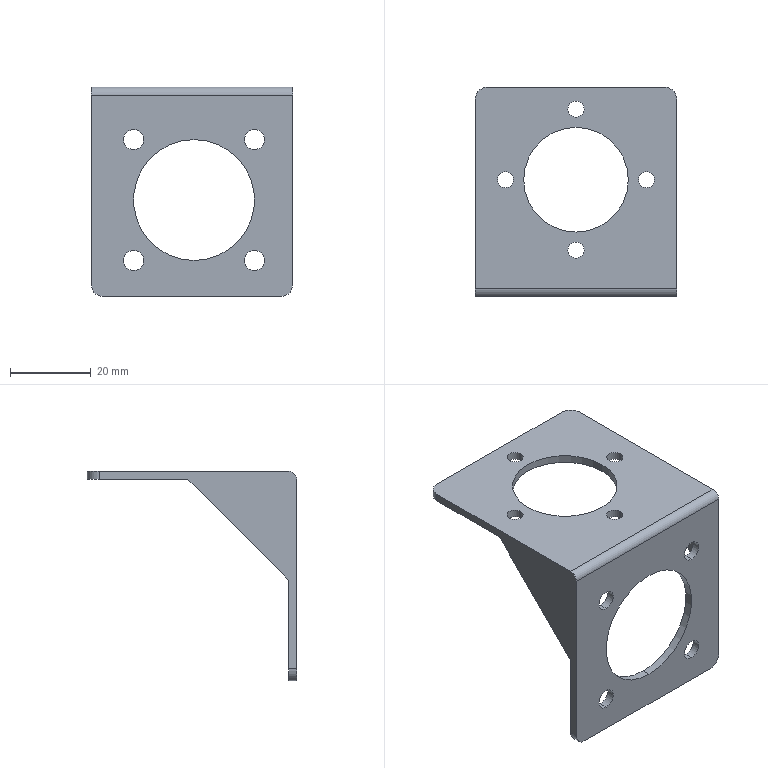Part | SolidWorks | features BaseBody 1 | 1 solid | 37 faces | box 50 x 52 x 52 mm | volume 8658 mm3 | cylinder 25 | plane 12 | commonest cylinder face diameters 4 x9 5 x8 6 x4 26 x2 30 x2
STEP:
#1=CARTESIAN_POINT('',(55.639,29.003,-82.334));
#2=VERTEX_POINT('',#1);
#3=CARTESIAN_POINT('',(51.639,29.003,-82.334));
#4=VERTEX_POINT('',#3);
#5=CARTESIAN_POINT('',(53.639,29.003,-82.334));
#6=DIRECTION('',(0.,0.,-1.));
#7=DIRECTION('',(-1.,0.,0.));
#8=AXIS2_PLACEMENT_3D('',#5,#6,#7);
#9=CIRCLE('',#8,2.);
#10=EDGE_CURVE('',#2,#4,#9,.T.);
#11=ORIENTED_EDGE('',*,*,#10,.F.);
#12=CARTESIAN_POINT('',(55.639,29.003,-84.334));
#13=VERTEX_POINT('',#12);
#14=CARTESIAN_POINT('',(55.639,29.003,-82.334));
#15=DIRECTION('',(0.,0.,-1.));
#16=VECTOR('',#15,1000.);
#17=LINE('',#14,#16);
#18=EDGE_CURVE('',#2,#13,#17,.T.);
#19=ORIENTED_EDGE('',*,*,#18,.T.);
#20=CARTESIAN_POINT('',(51.639,29.003,-84.334));
#21=VERTEX_POINT('',#20);
#22=CARTESIAN_POINT('',(53.639,29.003,-84.334));
#23=DIRECTION('',(0.,0.,1.));
#24=DIRECTION('',(-1.,0.,0.));
#25=AXIS2_PLACEMENT_3D('',#22,#23,#24);
#26=CIRCLE('',#25,2.);
#27=EDGE_CURVE('',#21,#13,#26,.T.);
#28=ORIENTED_EDGE('',*,*,#27,.F.);
#29=CARTESIAN_POINT('',(51.639,29.003,-82.334));
#30=DIRECTION('',(0.,0.,-1.));
#31=VECTOR('',#30,1000.);
#32=LINE('',#29,#31);
#33=EDGE_CURVE('',#4,#21,#32,.T.);
#34=ORIENTED_EDGE('',*,*,#33,.F.);
#35=EDGE_LOOP('',(#11,#19,#28,#34));
#36=FACE_OUTER_BOUND('',#35,.T.);
#37=CARTESIAN_POINT('',(53.639,29.003,-82.334));
#38=DIRECTION('',(0.,0.,-1.));
#39=DIRECTION('',(-1.,0.,0.));
#40=AXIS2_PLACEMENT_3D('',#37,#38,#39);
#41=CYLINDRICAL_SURFACE('',#40,2.);
#42=ADVANCED_FACE('',(#36),#41,.F.);
#43=CARTESIAN_POINT('',(84.139,29.003,-82.334));
#44=VERTEX_POINT('',#43);
#45=CARTESIAN_POINT('',(58.139,29.003,-82.334));
#46=VERTEX_POINT('',#45);
#47=CARTESIAN_POINT('',(71.139,29.003,-82.334));
#48=DIRECTION('',(0.,0.,-1.));
#49=DIRECTION('',(-1.,0.,0.));
#50=AXIS2_PLACEMENT_3D('',#47,#48,#49);
#51=CIRCLE('',#50,13.);
#52=EDGE_CURVE('',#44,#46,#51,.T.);
#53=ORIENTED_EDGE('',*,*,#52,.F.);
#54=CARTESIAN_POINT('',(84.139,29.003,-84.334));
#55=VERTEX_POINT('',#54);
#56=CARTESIAN_POINT('',(84.139,29.003,-82.334));
#57=DIRECTION('',(0.,0.,-1.));
#58=VECTOR('',#57,1000.);
#59=LINE('',#56,#58);
#60=EDGE_CURVE('',#44,#55,#59,.T.);
#61=ORIENTED_EDGE('',*,*,#60,.T.);
#62=CARTESIAN_POINT('',(58.139,29.003,-84.334));
#63=VERTEX_POINT('',#62);
#64=CARTESIAN_POINT('',(71.139,29.003,-84.334));
#65=DIRECTION('',(0.,0.,1.));
#66=DIRECTION('',(-1.,0.,0.));
#67=AXIS2_PLACEMENT_3D('',#64,#65,#66);
#68=CIRCLE('',#67,13.);
#69=EDGE_CURVE('',#63,#55,#68,.T.);
#70=ORIENTED_EDGE('',*,*,#69,.F.);
#71=CARTESIAN_POINT('',(58.139,29.003,-82.334));
#72=DIRECTION('',(0.,0.,-1.));
#73=VECTOR('',#72,1000.);
#74=LINE('',#71,#73);
#75=EDGE_CURVE('',#46,#63,#74,.T.);
#76=ORIENTED_EDGE('',*,*,#75,.F.);
#77=EDGE_LOOP('',(#53,#61,#70,#76));
#78=FACE_OUTER_BOUND('',#77,.T.);
#79=CARTESIAN_POINT('',(71.139,29.003,-82.334));
#80=DIRECTION('',(0.,0.,-1.));
#81=DIRECTION('',(-1.,0.,0.));
#82=AXIS2_PLACEMENT_3D('',#79,#80,#81);
#83=CYLINDRICAL_SURFACE('',#82,13.);
#84=ADVANCED_FACE('',(#78),#83,.F.);
#85=CARTESIAN_POINT('',(90.639,29.003,-82.334));
#86=VERTEX_POINT('',#85);
#87=CARTESIAN_POINT('',(86.639,29.003,-82.334));
#88=VERTEX_POINT('',#87);
#89=CARTESIAN_POINT('',(88.639,29.003,-82.334));
#90=DIRECTION('',(0.,0.,-1.));
#91=DIRECTION('',(-1.,0.,0.));
#92=AXIS2_PLACEMENT_3D('',#89,#90,#91);
#93=CIRCLE('',#92,2.);
#94=EDGE_CURVE('',#86,#88,#93,.T.);
#95=ORIENTED_EDGE('',*,*,#94,.F.);
#96=CARTESIAN_POINT('',(90.639,29.003,-84.334));
#97=VERTEX_POINT('',#96);
#98=CARTESIAN_POINT('',(90.639,29.003,-82.334));
#99=DIRECTION('',(0.,0.,-1.));
#100=VECTOR('',#99,1000.);
#101=LINE('',#98,#100);
#102=EDGE_CURVE('',#86,#97,#101,.T.);
#103=ORIENTED_EDGE('',*,*,#102,.T.);
#104=CARTESIAN_POINT('',(86.639,29.003,-84.334));
#105=VERTEX_POINT('',#104);
#106=CARTESIAN_POINT('',(88.639,29.003,-84.334));
#107=DIRECTION('',(0.,0.,1.));
#108=DIRECTION('',(-1.,0.,0.));
#109=AXIS2_PLACEMENT_3D('',#106,#107,#108);
#110=CIRCLE('',#109,2.);
#111=EDGE_CURVE('',#105,#97,#110,.T.);
#112=ORIENTED_EDGE('',*,*,#111,.F.);
#113=CARTESIAN_POINT('',(86.639,29.003,-82.334));
#114=DIRECTION('',(0.,0.,-1.));
#115=VECTOR('',#114,1000.);
#116=LINE('',#113,#115);
#117=EDGE_CURVE('',#88,#105,#116,.T.);
#118=ORIENTED_EDGE('',*,*,#117,.F.);
#119=EDGE_LOOP('',(#95,#103,#112,#118));
#120=FACE_OUTER_BOUND('',#119,.T.);
#121=CARTESIAN_POINT('',(88.639,29.003,-82.334));
#122=DIRECTION('',(0.,0.,-1.));
#123=DIRECTION('',(-1.,0.,0.));
#124=AXIS2_PLACEMENT_3D('',#121,#122,#123);
#125=CYLINDRICAL_SURFACE('',#124,2.);
#126=ADVANCED_FACE('',(#120),#125,.F.);
#127=CARTESIAN_POINT('',(73.139,11.503,-82.334));
#128=VERTEX_POINT('',#127);
#129=CARTESIAN_POINT('',(69.139,11.503,-82.334));
#130=VERTEX_POINT('',#129);
#131=CARTESIAN_POINT('',(71.139,11.503,-82.334));
#132=DIRECTION('',(0.,0.,-1.));
#133=DIRECTION('',(-1.,0.,0.));
#134=AXIS2_PLACEMENT_3D('',#131,#132,#133);
#135=CIRCLE('',#134,2.);
#136=EDGE_CURVE('',#128,#130,#135,.T.);
#137=ORIENTED_EDGE('',*,*,#136,.F.);
#138=CARTESIAN_POINT('',(73.139,11.503,-84.334));
#139=VERTEX_POINT('',#138);
#140=CARTESIAN_POINT('',(73.139,11.503,-82.334));
#141=DIRECTION('',(0.,0.,-1.));
#142=VECTOR('',#141,1000.);
#143=LINE('',#140,#142);
#144=EDGE_CURVE('',#128,#139,#143,.T.);
#145=ORIENTED_EDGE('',*,*,#144,.T.);
#146=CARTESIAN_POINT('',(69.139,11.503,-84.334));
#147=VERTEX_POINT('',#146);
#148=CARTESIAN_POINT('',(71.139,11.503,-84.334));
#149=DIRECTION('',(0.,0.,1.));
#150=DIRECTION('',(-1.,0.,0.));
#151=AXIS2_PLACEMENT_3D('',#148,#149,#150);
#152=CIRCLE('',#151,2.);
#153=EDGE_CURVE('',#147,#139,#152,.T.);
#154=ORIENTED_EDGE('',*,*,#153,.F.);
#155=CARTESIAN_POINT('',(69.139,11.503,-82.334));
#156=DIRECTION('',(0.,0.,-1.));
#157=VECTOR('',#156,1000.);
#158=LINE('',#155,#157);
#159=EDGE_CURVE('',#130,#147,#158,.T.);
#160=ORIENTED_EDGE('',*,*,#159,.F.);
#161=EDGE_LOOP('',(#137,#145,#154,#160));
#162=FACE_OUTER_BOUND('',#161,.T.);
#163=CARTESIAN_POINT('',(71.139,11.503,-82.334));
#164=DIRECTION('',(0.,0.,-1.));
#165=DIRECTION('',(-1.,0.,0.));
#166=AXIS2_PLACEMENT_3D('',#163,#164,#165);
#167=CYLINDRICAL_SURFACE('',#166,2.);
#168=ADVANCED_FACE('',(#162),#167,.F.);
#169=CARTESIAN_POINT('',(73.139,46.503,-82.334));
#170=VERTEX_POINT('',#169);
#171=CARTESIAN_POINT('',(69.139,46.503,-82.334));
#172=VERTEX_POINT('',#171);
#173=CARTESIAN_POINT('',(71.139,46.503,-82.334));
#174=DIRECTION('',(0.,0.,-1.));
#175=DIRECTION('',(-1.,0.,0.));
#176=AXIS2_PLACEMENT_3D('',#173,#174,#175);
#177=CIRCLE('',#176,2.);
#178=EDGE_CURVE('',#170,#172,#177,.T.);
#179=ORIENTED_EDGE('',*,*,#178,.F.);
#180=CARTESIAN_POINT('',(73.139,46.503,-84.334));
#181=VERTEX_POINT('',#180);
#182=CARTESIAN_POINT('',(73.139,46.503,-82.334));
#183=DIRECTION('',(0.,0.,-1.));
#184=VECTOR('',#183,1000.);
#185=LINE('',#182,#184);
#186=EDGE_CURVE('',#170,#181,#185,.T.);
#187=ORIENTED_EDGE('',*,*,#186,.T.);
#188=CARTESIAN_POINT('',(69.139,46.503,-84.334));
#189=VERTEX_POINT('',#188);
#190=CARTESIAN_POINT('',(71.139,46.503,-84.334));
#191=DIRECTION('',(0.,0.,1.));
#192=DIRECTION('',(-1.,0.,0.));
#193=AXIS2_PLACEMENT_3D('',#190,#191,#192);
#194=CIRCLE('',#193,2.);
#195=EDGE_CURVE('',#189,#181,#194,.T.);
#196=ORIENTED_EDGE('',*,*,#195,.F.);
#197=CARTESIAN_POINT('',(69.139,46.503,-82.334));
#198=DIRECTION('',(0.,0.,-1.));
#199=VECTOR('',#198,1000.);
#200=LINE('',#197,#199);
#201=EDGE_CURVE('',#172,#189,#200,.T.);
#202=ORIENTED_EDGE('',*,*,#201,.F.);
#203=EDGE_LOOP('',(#179,#187,#196,#202));
#204=FACE_OUTER_BOUND('',#203,.T.);
#205=CARTESIAN_POINT('',(71.139,46.503,-82.334));
#206=DIRECTION('',(0.,0.,-1.));
#207=DIRECTION('',(-1.,0.,0.));
#208=AXIS2_PLACEMENT_3D('',#205,#206,#207);
#209=CYLINDRICAL_SURFACE('',#208,2.);
#210=ADVANCED_FACE('',(#204),#209,.F.);
#211=CARTESIAN_POINT('',(56.639,2.,-122.834));
#212=VERTEX_POINT('',#211);
#213=CARTESIAN_POINT('',(56.639,2.,-127.834));
#214=VERTEX_POINT('',#213);
#215=CARTESIAN_POINT('',(56.639,2.,-125.334));
#216=DIRECTION('',(0.,-1.,0.));
#217=DIRECTION('',(0.,0.,-1.));
#218=AXIS2_PLACEMENT_3D('',#215,#216,#217);
#219=CIRCLE('',#218,2.5);
#220=EDGE_CURVE('',#212,#214,#219,.T.);
#221=ORIENTED_EDGE('',*,*,#220,.F.);
#222=CARTESIAN_POINT('',(56.639,0.,-122.834));
#223=VERTEX_POINT('',#222);
#224=CARTESIAN_POINT('',(56.639,2.,-122.834));
#225=DIRECTION('',(0.,-1.,0.));
#226=VECTOR('',#225,1000.);
#227=LINE('',#224,#226);
#228=EDGE_CURVE('',#212,#223,#227,.T.);
#229=ORIENTED_EDGE('',*,*,#228,.T.);
#230=CARTESIAN_POINT('',(56.639,0.,-127.834));
#231=VERTEX_POINT('',#230);
#232=CARTESIAN_POINT('',(56.639,0.,-125.334));
#233=DIRECTION('',(0.,-1.,0.));
#234=DIRECTION('',(0.,0.,-1.));
#235=AXIS2_PLACEMENT_3D('',#232,#233,#234);
#236=CIRCLE('',#235,2.5);
#237=EDGE_CURVE('',#223,#231,#236,.T.);
#238=ORIENTED_EDGE('',*,*,#237,.T.);
#239=CARTESIAN_POINT('',(56.639,2.,-127.834));
#240=DIRECTION('',(0.,-1.,0.));
#241=VECTOR('',#240,1000.);
#242=LINE('',#239,#241);
#243=EDGE_CURVE('',#214,#231,#242,.T.);
#244=ORIENTED_EDGE('',*,*,#243,.F.);
#245=EDGE_LOOP('',(#221,#229,#238,#244));
#246=FACE_OUTER_BOUND('',#245,.T.);
#247=CARTESIAN_POINT('',(56.639,2.,-125.334));
#248=DIRECTION('',(0.,-1.,0.));
#249=DIRECTION('',(0.,0.,-1.));
#250=AXIS2_PLACEMENT_3D('',#247,#248,#249);
#251=CYLINDRICAL_SURFACE('',#250,2.5);
#252=ADVANCED_FACE('',(#246),#251,.F.);
#253=CARTESIAN_POINT('',(86.639,2.,-122.834));
#254=VERTEX_POINT('',#253);
#255=CARTESIAN_POINT('',(86.639,2.,-127.834));
#256=VERTEX_POINT('',#255);
#257=CARTESIAN_POINT('',(86.639,2.,-125.334));
#258=DIRECTION('',(0.,-1.,0.));
#259=DIRECTION('',(0.,0.,-1.));
#260=AXIS2_PLACEMENT_3D('',#257,#258,#259);
#261=CIRCLE('',#260,2.5);
#262=EDGE_CURVE('',#254,#256,#261,.T.);
#263=ORIENTED_EDGE('',*,*,#262,.F.);
#264=CARTESIAN_POINT('',(86.639,0.,-122.834));
#265=VERTEX_POINT('',#264);
#266=CARTESIAN_POINT('',(86.639,2.,-122.834));
#267=DIRECTION('',(0.,-1.,0.));
#268=VECTOR('',#267,1000.);
#269=LINE('',#266,#268);
#270=EDGE_CURVE('',#254,#265,#269,.T.);
#271=ORIENTED_EDGE('',*,*,#270,.T.);
#272=CARTESIAN_POINT('',(86.639,0.,-127.834));
#273=VERTEX_POINT('',#272);
#274=CARTESIAN_POINT('',(86.639,0.,-125.334));
#275=DIRECTION('',(0.,-1.,0.));
#276=DIRECTION('',(0.,0.,-1.));
#277=AXIS2_PLACEMENT_3D('',#274,#275,#276);
#278=CIRCLE('',#277,2.5);
#279=EDGE_CURVE('',#265,#273,#278,.T.);
#280=ORIENTED_EDGE('',*,*,#279,.T.);
#281=CARTESIAN_POINT('',(86.639,2.,-127.834));
#282=DIRECTION('',(0.,-1.,0.));
#283=VECTOR('',#282,1000.);
#284=LINE('',#281,#283);
#285=EDGE_CURVE('',#256,#273,#284,.T.);
#286=ORIENTED_EDGE('',*,*,#285,.F.);
#287=EDGE_LOOP('',(#263,#271,#280,#286));
#288=FACE_OUTER_BOUND('',#287,.T.);
#289=CARTESIAN_POINT('',(86.639,2.,-125.334));
#290=DIRECTION('',(0.,-1.,0.));
#291=DIRECTION('',(0.,0.,-1.));
#292=AXIS2_PLACEMENT_3D('',#289,#290,#291);
#293=CYLINDRICAL_SURFACE('',#292,2.5);
#294=ADVANCED_FACE('',(#288),#293,.F.);
#295=CARTESIAN_POINT('',(56.639,2.,-92.834));
#296=VERTEX_POINT('',#295);
#297=CARTESIAN_POINT('',(56.639,2.,-97.834));
#298=VERTEX_POINT('',#297);
#299=CARTESIAN_POINT('',(56.639,2.,-95.334));
#300=DIRECTION('',(0.,-1.,0.));
#301=DIRECTION('',(0.,0.,-1.));
#302=AXIS2_PLACEMENT_3D('',#299,#300,#301);
#303=CIRCLE('',#302,2.5);
#304=EDGE_CURVE('',#296,#298,#303,.T.);
#305=ORIENTED_EDGE('',*,*,#304,.F.);
#306=CARTESIAN_POINT('',(56.639,0.,-92.834));
#307=VERTEX_POINT('',#306);
#308=CARTESIAN_POINT('',(56.639,2.,-92.834));
#309=DIRECTION('',(0.,-1.,0.));
#310=VECTOR('',#309,1000.);
#311=LINE('',#308,#310);
#312=EDGE_CURVE('',#296,#307,#311,.T.);
#313=ORIENTED_EDGE('',*,*,#312,.T.);
#314=CARTESIAN_POINT('',(56.639,0.,-97.834));
#315=VERTEX_POINT('',#314);
#316=CARTESIAN_POINT('',(56.639,0.,-95.334));
#317=DIRECTION('',(0.,-1.,0.));
#318=DIRECTION('',(0.,0.,-1.));
#319=AXIS2_PLACEMENT_3D('',#316,#317,#318);
#320=CIRCLE('',#319,2.5);
#321=EDGE_CURVE('',#307,#315,#320,.T.);
#322=ORIENTED_EDGE('',*,*,#321,.T.);
#323=CARTESIAN_POINT('',(56.639,2.,-97.834));
#324=DIRECTION('',(0.,-1.,0.));
#325=VECTOR('',#324,1000.);
#326=LINE('',#323,#325);
#327=EDGE_CURVE('',#298,#315,#326,.T.);
#328=ORIENTED_EDGE('',*,*,#327,.F.);
#329=EDGE_LOOP('',(#305,#313,#322,#328));
#330=FACE_OUTER_BOUND('',#329,.T.);
#331=CARTESIAN_POINT('',(56.639,2.,-95.334));
#332=DIRECTION('',(0.,-1.,0.));
#333=DIRECTION('',(0.,0.,-1.));
#334=AXIS2_PLACEMENT_3D('',#331,#332,#333);
#335=CYLINDRICAL_SURFACE('',#334,2.5);
#336=ADVANCED_FACE('',(#330),#335,.F.);
#337=CARTESIAN_POINT('',(86.639,2.,-92.834));
#338=VERTEX_POINT('',#337);
#339=CARTESIAN_POINT('',(86.639,2.,-97.834));
#340=VERTEX_POINT('',#339);
#341=CARTESIAN_POINT('',(86.639,2.,-95.334));
#342=DIRECTION('',(0.,-1.,0.));
#343=DIRECTION('',(0.,0.,-1.));
#344=AXIS2_PLACEMENT_3D('',#341,#342,#343);
#345=CIRCLE('',#344,2.5);
#346=EDGE_CURVE('',#338,#340,#345,.T.);
#347=ORIENTED_EDGE('',*,*,#346,.F.);
#348=CARTESIAN_POINT('',(86.639,0.,-92.834));
#349=VERTEX_POINT('',#348);
#350=CARTESIAN_POINT('',(86.639,2.,-92.834));
#351=DIRECTION('',(0.,-1.,0.));
#352=VECTOR('',#351,1000.);
#353=LINE('',#350,#352);
#354=EDGE_CURVE('',#338,#349,#353,.T.);
#355=ORIENTED_EDGE('',*,*,#354,.T.);
#356=CARTESIAN_POINT('',(86.639,0.,-97.834));
#357=VERTEX_POINT('',#356);
#358=CARTESIAN_POINT('',(86.639,0.,-95.334));
#359=DIRECTION('',(0.,-1.,0.));
#360=DIRECTION('',(0.,0.,-1.));
#361=AXIS2_PLACEMENT_3D('',#358,#359,#360);
#362=CIRCLE('',#361,2.5);
#363=EDGE_CURVE('',#349,#357,#362,.T.);
#364=ORIENTED_EDGE('',*,*,#363,.T.);
#365=CARTESIAN_POINT('',(86.639,2.,-97.834));
#366=DIRECTION('',(0.,-1.,0.));
#367=VECTOR('',#366,1000.);
#368=LINE('',#365,#367);
#369=EDGE_CURVE('',#340,#357,#368,.T.);
#370=ORIENTED_EDGE('',*,*,#369,.F.);
#371=EDGE_LOOP('',(#347,#355,#364,#370));
#372=FACE_OUTER_BOUND('',#371,.T.);
#373=CARTESIAN_POINT('',(86.639,2.,-95.334));
#374=DIRECTION('',(0.,-1.,0.));
#375=DIRECTION('',(0.,0.,-1.));
#376=AXIS2_PLACEMENT_3D('',#373,#374,#375);
#377=CYLINDRICAL_SURFACE('',#376,2.5);
#378=ADVANCED_FACE('',(#372),#377,.F.);
#379=CARTESIAN_POINT('',(71.639,2.,-95.334));
#380=VERTEX_POINT('',#379);
#381=CARTESIAN_POINT('',(71.639,2.,-125.334));
#382=VERTEX_POINT('',#381);
#383=CARTESIAN_POINT('',(71.639,2.,-110.334));
#384=DIRECTION('',(0.,-1.,0.));
#385=DIRECTION('',(0.,0.,-1.));
#386=AXIS2_PLACEMENT_3D('',#383,#384,#385);
#387=CIRCLE('',#386,15.);
#388=EDGE_CURVE('',#380,#382,#387,.T.);
#389=ORIENTED_EDGE('',*,*,#388,.F.);
#390=CARTESIAN_POINT('',(71.639,0.,-95.334));
#391=VERTEX_POINT('',#390);
#392=CARTESIAN_POINT('',(71.639,2.,-95.334));
#393=DIRECTION('',(0.,-1.,0.));
#394=VECTOR('',#393,1000.);
#395=LINE('',#392,#394);
#396=EDGE_CURVE('',#380,#391,#395,.T.);
#397=ORIENTED_EDGE('',*,*,#396,.T.);
#398=CARTESIAN_POINT('',(71.639,0.,-125.334));
#399=VERTEX_POINT('',#398);
#400=CARTESIAN_POINT('',(71.639,0.,-110.334));
#401=DIRECTION('',(0.,-1.,0.));
#402=DIRECTION('',(0.,0.,-1.));
#403=AXIS2_PLACEMENT_3D('',#400,#401,#402);
#404=CIRCLE('',#403,15.);
#405=EDGE_CURVE('',#391,#399,#404,.T.);
#406=ORIENTED_EDGE('',*,*,#405,.T.);
#407=CARTESIAN_POINT('',(71.639,2.,-125.334));
#408=DIRECTION('',(0.,-1.,0.));
#409=VECTOR('',#408,1000.);
#410=LINE('',#407,#409);
#411=EDGE_CURVE('',#382,#399,#410,.T.);
#412=ORIENTED_EDGE('',*,*,#411,.F.);
#413=EDGE_LOOP('',(#389,#397,#406,#412));
#414=FACE_OUTER_BOUND('',#413,.T.);
#415=CARTESIAN_POINT('',(71.639,2.,-110.334));
#416=DIRECTION('',(0.,-1.,0.));
#417=DIRECTION('',(0.,0.,-1.));
#418=AXIS2_PLACEMENT_3D('',#415,#416,#417);
#419=CYLINDRICAL_SURFACE('',#418,15.);
#420=ADVANCED_FACE('',(#414),#419,.F.);
#421=CARTESIAN_POINT('',(53.639,29.003,-82.334));
#422=DIRECTION('',(0.,0.,-1.));
#423=DIRECTION('',(-1.,0.,0.));
#424=AXIS2_PLACEMENT_3D('',#421,#422,#423);
#425=CIRCLE('',#424,2.);
#426=EDGE_CURVE('',#4,#2,#425,.T.);
#427=ORIENTED_EDGE('',*,*,#426,.T.);
#428=ORIENTED_EDGE('',*,*,#10,.T.);
#429=EDGE_LOOP('',(#427,#428));
#430=FACE_BOUND('',#429,.T.);
#431=CARTESIAN_POINT('',(71.139,29.003,-82.334));
#432=DIRECTION('',(0.,0.,-1.));
#433=DIRECTION('',(-1.,0.,0.));
#434=AXIS2_PLACEMENT_3D('',#431,#432,#433);
#435=CIRCLE('',#434,13.);
#436=EDGE_CURVE('',#46,#44,#435,.T.);
#437=ORIENTED_EDGE('',*,*,#436,.T.);
#438=ORIENTED_EDGE('',*,*,#52,.T.);
#439=EDGE_LOOP('',(#437,#438));
#440=FACE_BOUND('',#439,.T.);
#441=CARTESIAN_POINT('',(96.139,49.,-82.334));
#442=VERTEX_POINT('',#441);
#443=CARTESIAN_POINT('',(93.139,52.,-82.334));
#444=VERTEX_POINT('',#443);
#445=CARTESIAN_POINT('',(93.139,49.,-82.334));
#446=DIRECTION('',(0.,0.,1.));
#447=DIRECTION('',(-1.,0.,0.));
#448=AXIS2_PLACEMENT_3D('',#445,#446,#447);
#449=CIRCLE('',#448,3.);
#450=EDGE_CURVE('',#442,#444,#449,.T.);
#451=ORIENTED_EDGE('',*,*,#450,.T.);
#452=CARTESIAN_POINT('',(49.139,52.,-82.334));
#453=VERTEX_POINT('',#452);
#454=CARTESIAN_POINT('',(93.139,52.,-82.334));
#455=DIRECTION('',(-1.,0.,0.));
#456=VECTOR('',#455,1000.);
#457=LINE('',#454,#456);
#458=EDGE_CURVE('',#444,#453,#457,.T.);
#459=ORIENTED_EDGE('',*,*,#458,.T.);
#460=CARTESIAN_POINT('',(46.139,49.,-82.334));
#461=VERTEX_POINT('',#460);
#462=CARTESIAN_POINT('',(49.139,49.,-82.334));
#463=DIRECTION('',(0.,0.,1.));
#464=DIRECTION('',(-1.,0.,0.));
#465=AXIS2_PLACEMENT_3D('',#462,#463,#464);
#466=CIRCLE('',#465,3.);
#467=EDGE_CURVE('',#453,#461,#466,.T.);
#468=ORIENTED_EDGE('',*,*,#467,.T.);
#469=CARTESIAN_POINT('',(46.139,2.,-82.334));
#470=VERTEX_POINT('',#469);
#471=CARTESIAN_POINT('',(46.139,49.,-82.334));
#472=DIRECTION('',(0.,-1.,0.));
#473=VECTOR('',#472,1000.);
#474=LINE('',#471,#473);
#475=EDGE_CURVE('',#461,#470,#474,.T.);
#476=ORIENTED_EDGE('',*,*,#475,.T.);
#477=CARTESIAN_POINT('',(96.139,2.,-82.334));
#478=VERTEX_POINT('',#477);
#479=CARTESIAN_POINT('',(93.139,2.,-82.334));
#480=DIRECTION('',(1.,0.,0.));
#481=VECTOR('',#480,1000.);
#482=LINE('',#479,#481);
#483=EDGE_CURVE('',#470,#478,#482,.T.);
#484=ORIENTED_EDGE('',*,*,#483,.T.);
#485=CARTESIAN_POINT('',(96.139,49.,-82.334));
#486=DIRECTION('',(0.,1.,0.));
#487=VECTOR('',#486,1000.);
#488=LINE('',#485,#487);
#489=EDGE_CURVE('',#478,#442,#488,.T.);
#490=ORIENTED_EDGE('',*,*,#489,.T.);
#491=EDGE_LOOP('',(#451,#459,#468,#476,#484,#490));
#492=FACE_OUTER_BOUND('',#491,.T.);
#493=CARTESIAN_POINT('',(88.639,29.003,-82.334));
#494=DIRECTION('',(0.,0.,-1.));
#495=DIRECTION('',(-1.,0.,0.));
#496=AXIS2_PLACEMENT_3D('',#493,#494,#495);
#497=CIRCLE('',#496,2.);
#498=EDGE_CURVE('',#88,#86,#497,.T.);
#499=ORIENTED_EDGE('',*,*,#498,.T.);
#500=ORIENTED_EDGE('',*,*,#94,.T.);
#501=EDGE_LOOP('',(#499,#500));
#502=FACE_BOUND('',#501,.T.);
#503=CARTESIAN_POINT('',(71.139,11.503,-82.334));
#504=DIRECTION('',(0.,0.,-1.));
#505=DIRECTION('',(-1.,0.,0.));
#506=AXIS2_PLACEMENT_3D('',#503,#504,#505);
#507=CIRCLE('',#506,2.);
#508=EDGE_CURVE('',#130,#128,#507,.T.);
#509=ORIENTED_EDGE('',*,*,#508,.T.);
#510=ORIENTED_EDGE('',*,*,#136,.T.);
#511=EDGE_LOOP('',(#509,#510));
#512=FACE_BOUND('',#511,.T.);
#513=CARTESIAN_POINT('',(71.139,46.503,-82.334));
#514=DIRECTION('',(0.,0.,-1.));
#515=DIRECTION('',(-1.,0.,0.));
#516=AXIS2_PLACEMENT_3D('',#513,#514,#515);
#517=CIRCLE('',#516,2.);
#518=EDGE_CURVE('',#172,#170,#517,.T.);
#519=ORIENTED_EDGE('',*,*,#518,.T.);
#520=ORIENTED_EDGE('',*,*,#178,.T.);
#521=EDGE_LOOP('',(#519,#520));
#522=FACE_BOUND('',#521,.T.);
#523=CARTESIAN_POINT('',(93.139,49.,-82.334));
#524=DIRECTION('',(0.,0.,1.));
#525=DIRECTION('',(1.,0.,0.));
#526=AXIS2_PLACEMENT_3D('',#523,#524,#525);
#527=PLANE('',#526);
#528=ADVANCED_FACE('',(#430,#440,#492,#502,#512,#522),#527,.T.);
#529=ORIENTED_EDGE('',*,*,#18,.F.);
#530=ORIENTED_EDGE('',*,*,#426,.F.);
#531=ORIENTED_EDGE('',*,*,#33,.T.);
#532=CARTESIAN_POINT('',(53.639,29.003,-84.334));
#533=DIRECTION('',(0.,0.,1.));
#534=DIRECTION('',(-1.,0.,0.));
#535=AXIS2_PLACEMENT_3D('',#532,#533,#534);
#536=CIRCLE('',#535,2.);
#537=EDGE_CURVE('',#13,#21,#536,.T.);
#538=ORIENTED_EDGE('',*,*,#537,.F.);
#539=EDGE_LOOP('',(#529,#530,#531,#538));
#540=FACE_OUTER_BOUND('',#539,.T.);
#541=CARTESIAN_POINT('',(53.639,29.003,-82.334));
#542=DIRECTION('',(0.,0.,-1.));
#543=DIRECTION('',(-1.,0.,0.));
#544=AXIS2_PLACEMENT_3D('',#541,#542,#543);
#545=CYLINDRICAL_SURFACE('',#544,2.);
#546=ADVANCED_FACE('',(#540),#545,.F.);
#547=ORIENTED_EDGE('',*,*,#60,.F.);
#548=ORIENTED_EDGE('',*,*,#436,.F.);
#549=ORIENTED_EDGE('',*,*,#75,.T.);
#550=CARTESIAN_POINT('',(71.139,29.003,-84.334));
#551=DIRECTION('',(0.,0.,1.));
#552=DIRECTION('',(-1.,0.,0.));
#553=AXIS2_PLACEMENT_3D('',#550,#551,#552);
#554=CIRCLE('',#553,13.);
#555=EDGE_CURVE('',#55,#63,#554,.T.);
#556=ORIENTED_EDGE('',*,*,#555,.F.);
#557=EDGE_LOOP('',(#547,#548,#549,#556));
#558=FACE_OUTER_BOUND('',#557,.T.);
#559=CARTESIAN_POINT('',(71.139,29.003,-82.334));
#560=DIRECTION('',(0.,0.,-1.));
#561=DIRECTION('',(-1.,0.,0.));
#562=AXIS2_PLACEMENT_3D('',#559,#560,#561);
#563=CYLINDRICAL_SURFACE('',#562,13.);
#564=ADVANCED_FACE('',(#558),#563,.F.);
#565=ORIENTED_EDGE('',*,*,#458,.F.);
#566=CARTESIAN_POINT('',(93.139,52.,-84.334));
#567=VERTEX_POINT('',#566);
#568=CARTESIAN_POINT('',(93.139,52.,-82.334));
#569=DIRECTION('',(0.,0.,1.));
#570=VECTOR('',#569,1000.);
#571=LINE('',#568,#570);
#572=EDGE_CURVE('',#567,#444,#571,.T.);
#573=ORIENTED_EDGE('',*,*,#572,.F.);
#574=CARTESIAN_POINT('',(49.139,52.,-84.334));
#575=VERTEX_POINT('',#574);
#576=CARTESIAN_POINT('',(93.139,52.,-84.334));
#577=DIRECTION('',(1.,0.,0.));
#578=VECTOR('',#577,1000.);
#579=LINE('',#576,#578);
#580=EDGE_CURVE('',#575,#567,#579,.T.);
#581=ORIENTED_EDGE('',*,*,#580,.F.);
#582=CARTESIAN_POINT('',(49.139,52.,-82.334));
#583=DIRECTION('',(0.,0.,-1.));
#584=VECTOR('',#583,1000.);
#585=LINE('',#582,#584);
#586=EDGE_CURVE('',#453,#575,#585,.T.);
#587=ORIENTED_EDGE('',*,*,#586,.F.);
#588=EDGE_LOOP('',(#565,#573,#581,#587));
#589=FACE_OUTER_BOUND('',#588,.T.);
#590=CARTESIAN_POINT('',(93.139,52.,-82.334));
#591=DIRECTION('',(0.,-1.,0.));
#592=DIRECTION('',(0.,0.,-1.));
#593=AXIS2_PLACEMENT_3D('',#590,#591,#592);
#594=PLANE('',#593);
#595=ADVANCED_FACE('',(#589),#594,.F.);
#596=CARTESIAN_POINT('',(96.139,49.,-84.334));
#597=VERTEX_POINT('',#596);
#598=CARTESIAN_POINT('',(93.139,49.,-84.334));
#599=DIRECTION('',(0.,0.,1.));
#600=DIRECTION('',(-1.,0.,0.));
#601=AXIS2_PLACEMENT_3D('',#598,#599,#600);
#602=CIRCLE('',#601,3.);
#603=EDGE_CURVE('',#597,#567,#602,.T.);
#604=ORIENTED_EDGE('',*,*,#603,.T.);
#605=ORIENTED_EDGE('',*,*,#572,.T.);
#606=ORIENTED_EDGE('',*,*,#450,.F.);
#607=CARTESIAN_POINT('',(96.139,49.,-82.334));
#608=DIRECTION('',(0.,0.,-1.));
#609=VECTOR('',#608,1000.);
#610=LINE('',#607,#609);
#611=EDGE_CURVE('',#442,#597,#610,.T.);
#612=ORIENTED_EDGE('',*,*,#611,.T.);
#613=EDGE_LOOP('',(#604,#605,#606,#612));
#614=FACE_OUTER_BOUND('',#613,.T.);
#615=CARTESIAN_POINT('',(93.139,49.,-82.334));
#616=DIRECTION('',(0.,0.,-1.));
#617=DIRECTION('',(-1.,0.,0.));
#618=AXIS2_PLACEMENT_3D('',#615,#616,#617);
#619=CYLINDRICAL_SURFACE('',#618,3.);
#620=ADVANCED_FACE('',(#614),#619,.T.);
#621=CARTESIAN_POINT('',(96.139,27.,-84.334));
#622=VERTEX_POINT('',#621);
#623=CARTESIAN_POINT('',(96.139,2.,-84.334));
#624=DIRECTION('',(0.,-1.,0.));
#625=VECTOR('',#624,1000.);
#626=LINE('',#623,#625);
#627=EDGE_CURVE('',#597,#622,#626,.T.);
#628=ORIENTED_EDGE('',*,*,#627,.F.);
#629=ORIENTED_EDGE('',*,*,#611,.F.);
#630=ORIENTED_EDGE('',*,*,#489,.F.);
#631=CARTESIAN_POINT('',(96.139,0.,-84.334));
#632=VERTEX_POINT('',#631);
#633=CARTESIAN_POINT('',(96.139,2.,-84.334));
#634=DIRECTION('',(-1.,0.,0.));
#635=DIRECTION('',(0.,0.,1.));
#636=AXIS2_PLACEMENT_3D('',#633,#634,#635);
#637=CIRCLE('',#636,2.);
#638=EDGE_CURVE('',#632,#478,#637,.T.);
#639=ORIENTED_EDGE('',*,*,#638,.F.);
#640=CARTESIAN_POINT('',(96.139,0.,-131.334));
#641=VERTEX_POINT('',#640);
#642=CARTESIAN_POINT('',(96.139,0.,-131.334));
#643=DIRECTION('',(0.,0.,1.));
#644=VECTOR('',#643,1000.);
#645=LINE('',#642,#644);
#646=EDGE_CURVE('',#641,#632,#645,.T.);
#647=ORIENTED_EDGE('',*,*,#646,.F.);
#648=CARTESIAN_POINT('',(96.139,2.,-131.334));
#649=VERTEX_POINT('',#648);
#650=CARTESIAN_POINT('',(96.139,2.,-131.334));
#651=DIRECTION('',(0.,-1.,0.));
#652=VECTOR('',#651,1000.);
#653=LINE('',#650,#652);
#654=EDGE_CURVE('',#649,#641,#653,.T.);
#655=ORIENTED_EDGE('',*,*,#654,.F.);
#656=CARTESIAN_POINT('',(96.139,2.,-109.334));
#657=VERTEX_POINT('',#656);
#658=CARTESIAN_POINT('',(96.139,2.,-131.334));
#659=DIRECTION('',(0.,0.,-1.));
#660=VECTOR('',#659,1000.);
#661=LINE('',#658,#660);
#662=EDGE_CURVE('',#657,#649,#661,.T.);
#663=ORIENTED_EDGE('',*,*,#662,.F.);
#664=CARTESIAN_POINT('',(96.139,27.,-84.334));
#665=DIRECTION('',(0.,-0.7071,-0.7071));
#666=VECTOR('',#665,1000.);
#667=LINE('',#664,#666);
#668=EDGE_CURVE('',#622,#657,#667,.T.);
#669=ORIENTED_EDGE('',*,*,#668,.F.);
#670=EDGE_LOOP('',(#628,#629,#630,#639,#647,#655,#663,#669));
#671=FACE_OUTER_BOUND('',#670,.T.);
#672=CARTESIAN_POINT('',(96.139,2.,-131.334));
#673=DIRECTION('',(-1.,0.,0.));
#674=DIRECTION('',(0.,0.,1.));
#675=AXIS2_PLACEMENT_3D('',#672,#673,#674);
#676=PLANE('',#675);
#677=ADVANCED_FACE('',(#671),#676,.F.);
#678=CARTESIAN_POINT('',(46.139,0.,-84.334));
#679=VERTEX_POINT('',#678);
#680=CARTESIAN_POINT('',(46.139,2.,-84.334));
#681=DIRECTION('',(1.,0.,0.));
#682=DIRECTION('',(0.,0.,1.));
#683=AXIS2_PLACEMENT_3D('',#680,#681,#682);
#684=CIRCLE('',#683,2.);
#685=EDGE_CURVE('',#470,#679,#684,.T.);
#686=ORIENTED_EDGE('',*,*,#685,.T.);
#687=CARTESIAN_POINT('',(96.139,0.,-84.334));
#688=DIRECTION('',(1.,0.,0.));
#689=VECTOR('',#688,1000.);
#690=LINE('',#687,#689);
#691=EDGE_CURVE('',#679,#632,#690,.T.);
#692=ORIENTED_EDGE('',*,*,#691,.T.);
#693=ORIENTED_EDGE('',*,*,#638,.T.);
#694=ORIENTED_EDGE('',*,*,#483,.F.);
#695=EDGE_LOOP('',(#686,#692,#693,#694));
#696=FACE_OUTER_BOUND('',#695,.T.);
#697=CARTESIAN_POINT('',(96.139,2.,-84.334));
#698=DIRECTION('',(-1.,0.,0.));
#699=DIRECTION('',(0.,0.,1.));
#700=AXIS2_PLACEMENT_3D('',#697,#698,#699);
#701=CYLINDRICAL_SURFACE('',#700,2.);
#702=ADVANCED_FACE('',(#696),#701,.T.);
#703=ORIENTED_EDGE('',*,*,#475,.F.);
#704=CARTESIAN_POINT('',(46.139,49.,-84.334));
#705=VERTEX_POINT('',#704);
#706=CARTESIAN_POINT('',(46.139,49.,-84.334));
#707=DIRECTION('',(0.,0.,1.));
#708=VECTOR('',#707,1000.);
#709=LINE('',#706,#708);
#710=EDGE_CURVE('',#705,#461,#709,.T.);
#711=ORIENTED_EDGE('',*,*,#710,.F.);
#712=CARTESIAN_POINT('',(46.139,27.,-84.334));
#713=VERTEX_POINT('',#712);
#714=CARTESIAN_POINT('',(46.139,2.,-84.334));
#715=DIRECTION('',(0.,1.,0.));
#716=VECTOR('',#715,1000.);
#717=LINE('',#714,#716);
#718=EDGE_CURVE('',#713,#705,#717,.T.);
#719=ORIENTED_EDGE('',*,*,#718,.F.);
#720=CARTESIAN_POINT('',(46.139,2.,-109.334));
#721=VERTEX_POINT('',#720);
#722=CARTESIAN_POINT('',(46.139,2.,-109.334));
#723=DIRECTION('',(0.,0.7071,0.7071));
#724=VECTOR('',#723,1000.);
#725=LINE('',#722,#724);
#726=EDGE_CURVE('',#721,#713,#725,.T.);
#727=ORIENTED_EDGE('',*,*,#726,.F.);
#728=CARTESIAN_POINT('',(46.139,2.,-131.334));
#729=VERTEX_POINT('',#728);
#730=CARTESIAN_POINT('',(46.139,2.,-84.334));
#731=DIRECTION('',(0.,0.,1.));
#732=VECTOR('',#731,1000.);
#733=LINE('',#730,#732);
#734=EDGE_CURVE('',#729,#721,#733,.T.);
#735=ORIENTED_EDGE('',*,*,#734,.F.);
#736=CARTESIAN_POINT('',(46.139,0.,-131.334));
#737=VERTEX_POINT('',#736);
#738=CARTESIAN_POINT('',(46.139,2.,-131.334));
#739=DIRECTION('',(0.,1.,0.));
#740=VECTOR('',#739,1000.);
#741=LINE('',#738,#740);
#742=EDGE_CURVE('',#737,#729,#741,.T.);
#743=ORIENTED_EDGE('',*,*,#742,.F.);
#744=CARTESIAN_POINT('',(46.139,0.,-84.334));
#745=DIRECTION('',(0.,0.,-1.));
#746=VECTOR('',#745,1000.);
#747=LINE('',#744,#746);
#748=EDGE_CURVE('',#679,#737,#747,.T.);
#749=ORIENTED_EDGE('',*,*,#748,.F.);
#750=ORIENTED_EDGE('',*,*,#685,.F.);
#751=EDGE_LOOP('',(#703,#711,#719,#727,#735,#743,#749,#750));
#752=FACE_OUTER_BOUND('',#751,.T.);
#753=CARTESIAN_POINT('',(46.139,2.,-84.334));
#754=DIRECTION('',(1.,0.,0.));
#755=DIRECTION('',(0.,0.,-1.));
#756=AXIS2_PLACEMENT_3D('',#753,#754,#755);
#757=PLANE('',#756);
#758=ADVANCED_FACE('',(#752),#757,.F.);
#759=CARTESIAN_POINT('',(49.139,49.,-84.334));
#760=DIRECTION('',(0.,0.,1.));
#761=DIRECTION('',(-1.,0.,0.));
#762=AXIS2_PLACEMENT_3D('',#759,#760,#761);
#763=CIRCLE('',#762,3.);
#764=EDGE_CURVE('',#575,#705,#763,.T.);
#765=ORIENTED_EDGE('',*,*,#764,.T.);
#766=ORIENTED_EDGE('',*,*,#710,.T.);
#767=ORIENTED_EDGE('',*,*,#467,.F.);
#768=ORIENTED_EDGE('',*,*,#586,.T.);
#769=EDGE_LOOP('',(#765,#766,#767,#768));
#770=FACE_OUTER_BOUND('',#769,.T.);
#771=CARTESIAN_POINT('',(49.139,49.,-82.334));
#772=DIRECTION('',(0.,0.,-1.));
#773=DIRECTION('',(-1.,0.,0.));
#774=AXIS2_PLACEMENT_3D('',#771,#772,#773);
#775=CYLINDRICAL_SURFACE('',#774,3.);
#776=ADVANCED_FACE('',(#770),#775,.T.);
#777=ORIENTED_EDGE('',*,*,#102,.F.);
#778=ORIENTED_EDGE('',*,*,#498,.F.);
#779=ORIENTED_EDGE('',*,*,#117,.T.);
#780=CARTESIAN_POINT('',(88.639,29.003,-84.334));
#781=DIRECTION('',(0.,0.,1.));
#782=DIRECTION('',(-1.,0.,0.));
#783=AXIS2_PLACEMENT_3D('',#780,#781,#782);
#784=CIRCLE('',#783,2.);
#785=EDGE_CURVE('',#97,#105,#784,.T.);
#786=ORIENTED_EDGE('',*,*,#785,.F.);
#787=EDGE_LOOP('',(#777,#778,#779,#786));
#788=FACE_OUTER_BOUND('',#787,.T.);
#789=CARTESIAN_POINT('',(88.639,29.003,-82.334));
#790=DIRECTION('',(0.,0.,-1.));
#791=DIRECTION('',(-1.,0.,0.));
#792=AXIS2_PLACEMENT_3D('',#789,#790,#791);
#793=CYLINDRICAL_SURFACE('',#792,2.);
#794=ADVANCED_FACE('',(#788),#793,.F.);
#795=ORIENTED_EDGE('',*,*,#144,.F.);
#796=ORIENTED_EDGE('',*,*,#508,.F.);
#797=ORIENTED_EDGE('',*,*,#159,.T.);
#798=CARTESIAN_POINT('',(71.139,11.503,-84.334));
#799=DIRECTION('',(0.,0.,1.));
#800=DIRECTION('',(-1.,0.,0.));
#801=AXIS2_PLACEMENT_3D('',#798,#799,#800);
#802=CIRCLE('',#801,2.);
#803=EDGE_CURVE('',#139,#147,#802,.T.);
#804=ORIENTED_EDGE('',*,*,#803,.F.);
#805=EDGE_LOOP('',(#795,#796,#797,#804));
#806=FACE_OUTER_BOUND('',#805,.T.);
#807=CARTESIAN_POINT('',(71.139,11.503,-82.334));
#808=DIRECTION('',(0.,0.,-1.));
#809=DIRECTION('',(-1.,0.,0.));
#810=AXIS2_PLACEMENT_3D('',#807,#808,#809);
#811=CYLINDRICAL_SURFACE('',#810,2.);
#812=ADVANCED_FACE('',(#806),#811,.F.);
#813=ORIENTED_EDGE('',*,*,#186,.F.);
#814=ORIENTED_EDGE('',*,*,#518,.F.);
#815=ORIENTED_EDGE('',*,*,#201,.T.);
#816=CARTESIAN_POINT('',(71.139,46.503,-84.334));
#817=DIRECTION('',(0.,0.,1.));
#818=DIRECTION('',(-1.,0.,0.));
#819=AXIS2_PLACEMENT_3D('',#816,#817,#818);
#820=CIRCLE('',#819,2.);
#821=EDGE_CURVE('',#181,#189,#820,.T.);
#822=ORIENTED_EDGE('',*,*,#821,.F.);
#823=EDGE_LOOP('',(#813,#814,#815,#822));
#824=FACE_OUTER_BOUND('',#823,.T.);
#825=CARTESIAN_POINT('',(71.139,46.503,-82.334));
#826=DIRECTION('',(0.,0.,-1.));
#827=DIRECTION('',(-1.,0.,0.));
#828=AXIS2_PLACEMENT_3D('',#825,#826,#827);
#829=CYLINDRICAL_SURFACE('',#828,2.);
#830=ADVANCED_FACE('',(#824),#829,.F.);
#831=CARTESIAN_POINT('',(94.139,2.,-84.334));
#832=VERTEX_POINT('',#831);
#833=CARTESIAN_POINT('',(94.139,27.,-84.334));
#834=VERTEX_POINT('',#833);
#835=CARTESIAN_POINT('',(94.139,49.,-84.334));
#836=DIRECTION('',(0.,1.,0.));
#837=VECTOR('',#836,1000.);
#838=LINE('',#835,#837);
#839=EDGE_CURVE('',#832,#834,#838,.T.);
#840=ORIENTED_EDGE('',*,*,#839,.F.);
#841=CARTESIAN_POINT('',(48.139,2.,-84.334));
#842=VERTEX_POINT('',#841);
#843=CARTESIAN_POINT('',(93.139,2.,-84.334));
#844=DIRECTION('',(1.,0.,0.));
#845=VECTOR('',#844,1000.);
#846=LINE('',#843,#845);
#847=EDGE_CURVE('',#842,#832,#846,.T.);
#848=ORIENTED_EDGE('',*,*,#847,.F.);
#849=CARTESIAN_POINT('',(48.139,27.,-84.334));
#850=VERTEX_POINT('',#849);
#851=CARTESIAN_POINT('',(48.139,49.,-84.334));
#852=DIRECTION('',(0.,-1.,0.));
#853=VECTOR('',#852,1000.);
#854=LINE('',#851,#853);
#855=EDGE_CURVE('',#850,#842,#854,.T.);
#856=ORIENTED_EDGE('',*,*,#855,.F.);
#857=CARTESIAN_POINT('',(93.139,27.,-84.334));
#858=DIRECTION('',(1.,0.,0.));
#859=VECTOR('',#858,1000.);
#860=LINE('',#857,#859);
#861=EDGE_CURVE('',#713,#850,#860,.T.);
#862=ORIENTED_EDGE('',*,*,#861,.F.);
#863=ORIENTED_EDGE('',*,*,#718,.T.);
#864=ORIENTED_EDGE('',*,*,#764,.F.);
#865=ORIENTED_EDGE('',*,*,#580,.T.);
#866=ORIENTED_EDGE('',*,*,#603,.F.);
#867=ORIENTED_EDGE('',*,*,#627,.T.);
#868=CARTESIAN_POINT('',(93.139,27.,-84.334));
#869=DIRECTION('',(1.,0.,0.));
#870=VECTOR('',#869,1000.);
#871=LINE('',#868,#870);
#872=EDGE_CURVE('',#834,#622,#871,.T.);
#873=ORIENTED_EDGE('',*,*,#872,.F.);
#874=EDGE_LOOP('',(#840,#848,#856,#862,#863,#864,#865,#866,#867,#873));
#875=FACE_OUTER_BOUND('',#874,.T.);
#876=ORIENTED_EDGE('',*,*,#111,.T.);
#877=ORIENTED_EDGE('',*,*,#785,.T.);
#878=EDGE_LOOP('',(#876,#877));
#879=FACE_BOUND('',#878,.T.);
#880=ORIENTED_EDGE('',*,*,#69,.T.);
#881=ORIENTED_EDGE('',*,*,#555,.T.);
#882=EDGE_LOOP('',(#880,#881));
#883=FACE_BOUND('',#882,.T.);
#884=ORIENTED_EDGE('',*,*,#153,.T.);
#885=ORIENTED_EDGE('',*,*,#803,.T.);
#886=EDGE_LOOP('',(#884,#885));
#887=FACE_BOUND('',#886,.T.);
#888=ORIENTED_EDGE('',*,*,#27,.T.);
#889=ORIENTED_EDGE('',*,*,#537,.T.);
#890=EDGE_LOOP('',(#888,#889));
#891=FACE_BOUND('',#890,.T.);
#892=ORIENTED_EDGE('',*,*,#195,.T.);
#893=ORIENTED_EDGE('',*,*,#821,.T.);
#894=EDGE_LOOP('',(#892,#893));
#895=FACE_BOUND('',#894,.T.);
#896=CARTESIAN_POINT('',(93.139,49.,-84.334));
#897=DIRECTION('',(0.,0.,1.));
#898=DIRECTION('',(1.,0.,0.));
#899=AXIS2_PLACEMENT_3D('',#896,#897,#898);
#900=PLANE('',#899);
#901=ADVANCED_FACE('',(#875,#879,#883,#887,#891,#895),#900,.F.);
#902=ORIENTED_EDGE('',*,*,#668,.T.);
#903=CARTESIAN_POINT('',(94.139,2.,-109.334));
#904=VERTEX_POINT('',#903);
#905=CARTESIAN_POINT('',(94.139,2.,-109.334));
#906=DIRECTION('',(-1.,0.,0.));
#907=VECTOR('',#906,1000.);
#908=LINE('',#905,#907);
#909=EDGE_CURVE('',#657,#904,#908,.T.);
#910=ORIENTED_EDGE('',*,*,#909,.T.);
#911=CARTESIAN_POINT('',(94.139,27.,-84.334));
#912=DIRECTION('',(0.,0.7071,0.7071));
#913=VECTOR('',#912,1000.);
#914=LINE('',#911,#913);
#915=EDGE_CURVE('',#904,#834,#914,.T.);
#916=ORIENTED_EDGE('',*,*,#915,.T.);
#917=ORIENTED_EDGE('',*,*,#872,.T.);
#918=EDGE_LOOP('',(#902,#910,#916,#917));
#919=FACE_OUTER_BOUND('',#918,.T.);
#920=CARTESIAN_POINT('',(94.139,27.,-84.334));
#921=DIRECTION('',(0.,0.7071,-0.7071));
#922=DIRECTION('',(0.,0.7071,0.7071));
#923=AXIS2_PLACEMENT_3D('',#920,#921,#922);
#924=PLANE('',#923);
#925=ADVANCED_FACE('',(#919),#924,.T.);
#926=CARTESIAN_POINT('',(49.139,0.,-134.334));
#927=VERTEX_POINT('',#926);
#928=CARTESIAN_POINT('',(49.139,0.,-131.334));
#929=DIRECTION('',(0.,1.,0.));
#930=DIRECTION('',(0.,0.,-1.));
#931=AXIS2_PLACEMENT_3D('',#928,#929,#930);
#932=CIRCLE('',#931,3.);
#933=EDGE_CURVE('',#927,#737,#932,.T.);
#934=ORIENTED_EDGE('',*,*,#933,.F.);
#935=CARTESIAN_POINT('',(93.139,0.,-134.334));
#936=VERTEX_POINT('',#935);
#937=CARTESIAN_POINT('',(93.139,0.,-134.334));
#938=DIRECTION('',(-1.,0.,0.));
#939=VECTOR('',#938,1000.);
#940=LINE('',#937,#939);
#941=EDGE_CURVE('',#936,#927,#940,.T.);
#942=ORIENTED_EDGE('',*,*,#941,.F.);
#943=CARTESIAN_POINT('',(93.139,0.,-131.334));
#944=DIRECTION('',(0.,1.,0.));
#945=DIRECTION('',(0.,0.,-1.));
#946=AXIS2_PLACEMENT_3D('',#943,#944,#945);
#947=CIRCLE('',#946,3.);
#948=EDGE_CURVE('',#641,#936,#947,.T.);
#949=ORIENTED_EDGE('',*,*,#948,.F.);
#950=ORIENTED_EDGE('',*,*,#646,.T.);
#951=ORIENTED_EDGE('',*,*,#691,.F.);
#952=ORIENTED_EDGE('',*,*,#748,.T.);
#953=EDGE_LOOP('',(#934,#942,#949,#950,#951,#952));
#954=FACE_OUTER_BOUND('',#953,.T.);
#955=CARTESIAN_POINT('',(56.639,0.,-125.334));
#956=DIRECTION('',(0.,-1.,0.));
#957=DIRECTION('',(0.,0.,-1.));
#958=AXIS2_PLACEMENT_3D('',#955,#956,#957);
#959=CIRCLE('',#958,2.5);
#960=EDGE_CURVE('',#231,#223,#959,.T.);
#961=ORIENTED_EDGE('',*,*,#960,.F.);
#962=ORIENTED_EDGE('',*,*,#237,.F.);
#963=EDGE_LOOP('',(#961,#962));
#964=FACE_BOUND('',#963,.T.);
#965=CARTESIAN_POINT('',(86.639,0.,-125.334));
#966=DIRECTION('',(0.,-1.,0.));
#967=DIRECTION('',(0.,0.,-1.));
#968=AXIS2_PLACEMENT_3D('',#965,#966,#967);
#969=CIRCLE('',#968,2.5);
#970=EDGE_CURVE('',#273,#265,#969,.T.);
#971=ORIENTED_EDGE('',*,*,#970,.F.);
#972=ORIENTED_EDGE('',*,*,#279,.F.);
#973=EDGE_LOOP('',(#971,#972));
#974=FACE_BOUND('',#973,.T.);
#975=CARTESIAN_POINT('',(56.639,0.,-95.334));
#976=DIRECTION('',(0.,-1.,0.));
#977=DIRECTION('',(0.,0.,-1.));
#978=AXIS2_PLACEMENT_3D('',#975,#976,#977);
#979=CIRCLE('',#978,2.5);
#980=EDGE_CURVE('',#315,#307,#979,.T.);
#981=ORIENTED_EDGE('',*,*,#980,.F.);
#982=ORIENTED_EDGE('',*,*,#321,.F.);
#983=EDGE_LOOP('',(#981,#982));
#984=FACE_BOUND('',#983,.T.);
#985=CARTESIAN_POINT('',(86.639,0.,-95.334));
#986=DIRECTION('',(0.,-1.,0.));
#987=DIRECTION('',(0.,0.,-1.));
#988=AXIS2_PLACEMENT_3D('',#985,#986,#987);
#989=CIRCLE('',#988,2.5);
#990=EDGE_CURVE('',#357,#349,#989,.T.);
#991=ORIENTED_EDGE('',*,*,#990,.F.);
#992=ORIENTED_EDGE('',*,*,#363,.F.);
#993=EDGE_LOOP('',(#991,#992));
#994=FACE_BOUND('',#993,.T.);
#995=CARTESIAN_POINT('',(71.639,0.,-110.334));
#996=DIRECTION('',(0.,-1.,0.));
#997=DIRECTION('',(0.,0.,-1.));
#998=AXIS2_PLACEMENT_3D('',#995,#996,#997);
#999=CIRCLE('',#998,15.);
#1000=EDGE_CURVE('',#399,#391,#999,.T.);
#1001=ORIENTED_EDGE('',*,*,#1000,.F.);
#1002=ORIENTED_EDGE('',*,*,#405,.F.);
#1003=EDGE_LOOP('',(#1001,#1002));
#1004=FACE_BOUND('',#1003,.T.);
#1005=CARTESIAN_POINT('',(93.139,0.,-131.334));
#1006=DIRECTION('',(0.,1.,0.));
#1007=DIRECTION('',(0.,0.,1.));
#1008=AXIS2_PLACEMENT_3D('',#1005,#1006,#1007);
#1009=PLANE('',#1008);
#1010=ADVANCED_FACE('',(#954,#964,#974,#984,#994,#1004),#1009,.F.);
#1011=ORIENTED_EDGE('',*,*,#948,.T.);
#1012=CARTESIAN_POINT('',(93.139,2.,-134.334));
#1013=VERTEX_POINT('',#1012);
#1014=CARTESIAN_POINT('',(93.139,2.,-134.334));
#1015=DIRECTION('',(0.,1.,0.));
#1016=VECTOR('',#1015,1000.);
#1017=LINE('',#1014,#1016);
#1018=EDGE_CURVE('',#936,#1013,#1017,.T.);
#1019=ORIENTED_EDGE('',*,*,#1018,.T.);
#1020=CARTESIAN_POINT('',(93.139,2.,-131.334));
#1021=DIRECTION('',(0.,-1.,0.));
#1022=DIRECTION('',(0.,0.,-1.));
#1023=AXIS2_PLACEMENT_3D('',#1020,#1021,#1022);
#1024=CIRCLE('',#1023,3.);
#1025=EDGE_CURVE('',#1013,#649,#1024,.T.);
#1026=ORIENTED_EDGE('',*,*,#1025,.T.);
#1027=ORIENTED_EDGE('',*,*,#654,.T.);
#1028=EDGE_LOOP('',(#1011,#1019,#1026,#1027));
#1029=FACE_OUTER_BOUND('',#1028,.T.);
#1030=CARTESIAN_POINT('',(93.139,2.,-131.334));
#1031=DIRECTION('',(0.,-1.,0.));
#1032=DIRECTION('',(0.,0.,-1.));
#1033=AXIS2_PLACEMENT_3D('',#1030,#1031,#1032);
#1034=CYLINDRICAL_SURFACE('',#1033,3.);
#1035=ADVANCED_FACE('',(#1029),#1034,.T.);
#1036=CARTESIAN_POINT('',(48.139,2.,-109.334));
#1037=VERTEX_POINT('',#1036);
#1038=CARTESIAN_POINT('',(93.139,2.,-109.334));
#1039=DIRECTION('',(1.,0.,0.));
#1040=VECTOR('',#1039,1000.);
#1041=LINE('',#1038,#1040);
#1042=EDGE_CURVE('',#721,#1037,#1041,.T.);
#1043=ORIENTED_EDGE('',*,*,#1042,.T.);
#1044=CARTESIAN_POINT('',(48.139,2.,-131.334));
#1045=DIRECTION('',(0.,0.,1.));
#1046=VECTOR('',#1045,1000.);
#1047=LINE('',#1044,#1046);
#1048=EDGE_CURVE('',#1037,#842,#1047,.T.);
#1049=ORIENTED_EDGE('',*,*,#1048,.T.);
#1050=ORIENTED_EDGE('',*,*,#847,.T.);
#1051=CARTESIAN_POINT('',(94.139,2.,-131.334));
#1052=DIRECTION('',(0.,0.,-1.));
#1053=VECTOR('',#1052,1000.);
#1054=LINE('',#1051,#1053);
#1055=EDGE_CURVE('',#832,#904,#1054,.T.);
#1056=ORIENTED_EDGE('',*,*,#1055,.T.);
#1057=ORIENTED_EDGE('',*,*,#909,.F.);
#1058=ORIENTED_EDGE('',*,*,#662,.T.);
#1059=ORIENTED_EDGE('',*,*,#1025,.F.);
#1060=CARTESIAN_POINT('',(49.139,2.,-134.334));
#1061=VERTEX_POINT('',#1060);
#1062=CARTESIAN_POINT('',(93.139,2.,-134.334));
#1063=DIRECTION('',(-1.,0.,0.));
#1064=VECTOR('',#1063,1000.);
#1065=LINE('',#1062,#1064);
#1066=EDGE_CURVE('',#1013,#1061,#1065,.T.);
#1067=ORIENTED_EDGE('',*,*,#1066,.T.);
#1068=CARTESIAN_POINT('',(49.139,2.,-131.334));
#1069=DIRECTION('',(0.,1.,0.));
#1070=DIRECTION('',(0.,0.,-1.));
#1071=AXIS2_PLACEMENT_3D('',#1068,#1069,#1070);
#1072=CIRCLE('',#1071,3.);
#1073=EDGE_CURVE('',#1061,#729,#1072,.T.);
#1074=ORIENTED_EDGE('',*,*,#1073,.T.);
#1075=ORIENTED_EDGE('',*,*,#734,.T.);
#1076=EDGE_LOOP('',(#1043,#1049,#1050,#1056,#1057,#1058,#1059,#1067,#1074,#1075));
#1077=FACE_OUTER_BOUND('',#1076,.T.);
#1078=CARTESIAN_POINT('',(86.639,2.,-95.334));
#1079=DIRECTION('',(0.,-1.,0.));
#1080=DIRECTION('',(0.,0.,-1.));
#1081=AXIS2_PLACEMENT_3D('',#1078,#1079,#1080);
#1082=CIRCLE('',#1081,2.5);
#1083=EDGE_CURVE('',#340,#338,#1082,.T.);
#1084=ORIENTED_EDGE('',*,*,#1083,.T.);
#1085=ORIENTED_EDGE('',*,*,#346,.T.);
#1086=EDGE_LOOP('',(#1084,#1085));
#1087=FACE_BOUND('',#1086,.T.);
#1088=CARTESIAN_POINT('',(86.639,2.,-125.334));
#1089=DIRECTION('',(0.,-1.,0.));
#1090=DIRECTION('',(0.,0.,-1.));
#1091=AXIS2_PLACEMENT_3D('',#1088,#1089,#1090);
#1092=CIRCLE('',#1091,2.5);
#1093=EDGE_CURVE('',#256,#254,#1092,.T.);
#1094=ORIENTED_EDGE('',*,*,#1093,.T.);
#1095=ORIENTED_EDGE('',*,*,#262,.T.);
#1096=EDGE_LOOP('',(#1094,#1095));
#1097=FACE_BOUND('',#1096,.T.);
#1098=CARTESIAN_POINT('',(56.639,2.,-125.334));
#1099=DIRECTION('',(0.,-1.,0.));
#1100=DIRECTION('',(0.,0.,-1.));
#1101=AXIS2_PLACEMENT_3D('',#1098,#1099,#1100);
#1102=CIRCLE('',#1101,2.5);
#1103=EDGE_CURVE('',#214,#212,#1102,.T.);
#1104=ORIENTED_EDGE('',*,*,#1103,.T.);
#1105=ORIENTED_EDGE('',*,*,#220,.T.);
#1106=EDGE_LOOP('',(#1104,#1105));
#1107=FACE_BOUND('',#1106,.T.);
#1108=CARTESIAN_POINT('',(56.639,2.,-95.334));
#1109=DIRECTION('',(0.,-1.,0.));
#1110=DIRECTION('',(0.,0.,-1.));
#1111=AXIS2_PLACEMENT_3D('',#1108,#1109,#1110);
#1112=CIRCLE('',#1111,2.5);
#1113=EDGE_CURVE('',#298,#296,#1112,.T.);
#1114=ORIENTED_EDGE('',*,*,#1113,.T.);
#1115=ORIENTED_EDGE('',*,*,#304,.T.);
#1116=EDGE_LOOP('',(#1114,#1115));
#1117=FACE_BOUND('',#1116,.T.);
#1118=CARTESIAN_POINT('',(71.639,2.,-110.334));
#1119=DIRECTION('',(0.,-1.,0.));
#1120=DIRECTION('',(0.,0.,-1.));
#1121=AXIS2_PLACEMENT_3D('',#1118,#1119,#1120);
#1122=CIRCLE('',#1121,15.);
#1123=EDGE_CURVE('',#382,#380,#1122,.T.);
#1124=ORIENTED_EDGE('',*,*,#1123,.T.);
#1125=ORIENTED_EDGE('',*,*,#388,.T.);
#1126=EDGE_LOOP('',(#1124,#1125));
#1127=FACE_BOUND('',#1126,.T.);
#1128=CARTESIAN_POINT('',(93.139,2.,-131.334));
#1129=DIRECTION('',(0.,1.,0.));
#1130=DIRECTION('',(0.,0.,1.));
#1131=AXIS2_PLACEMENT_3D('',#1128,#1129,#1130);
#1132=PLANE('',#1131);
#1133=ADVANCED_FACE('',(#1077,#1087,#1097,#1107,#1117,#1127),#1132,.T.);
#1134=ORIENTED_EDGE('',*,*,#726,.T.);
#1135=ORIENTED_EDGE('',*,*,#861,.T.);
#1136=CARTESIAN_POINT('',(48.139,2.,-109.334));
#1137=DIRECTION('',(0.,-0.7071,-0.7071));
#1138=VECTOR('',#1137,1000.);
#1139=LINE('',#1136,#1138);
#1140=EDGE_CURVE('',#850,#1037,#1139,.T.);
#1141=ORIENTED_EDGE('',*,*,#1140,.T.);
#1142=ORIENTED_EDGE('',*,*,#1042,.F.);
#1143=EDGE_LOOP('',(#1134,#1135,#1141,#1142));
#1144=FACE_OUTER_BOUND('',#1143,.T.);
#1145=CARTESIAN_POINT('',(48.139,2.,-109.334));
#1146=DIRECTION('',(0.,0.7071,-0.7071));
#1147=DIRECTION('',(0.,0.7071,0.7071));
#1148=AXIS2_PLACEMENT_3D('',#1145,#1146,#1147);
#1149=PLANE('',#1148);
#1150=ADVANCED_FACE('',(#1144),#1149,.T.);
#1151=ORIENTED_EDGE('',*,*,#933,.T.);
#1152=ORIENTED_EDGE('',*,*,#742,.T.);
#1153=ORIENTED_EDGE('',*,*,#1073,.F.);
#1154=CARTESIAN_POINT('',(49.139,2.,-134.334));
#1155=DIRECTION('',(0.,-1.,0.));
#1156=VECTOR('',#1155,1000.);
#1157=LINE('',#1154,#1156);
#1158=EDGE_CURVE('',#1061,#927,#1157,.T.);
#1159=ORIENTED_EDGE('',*,*,#1158,.T.);
#1160=EDGE_LOOP('',(#1151,#1152,#1153,#1159));
#1161=FACE_OUTER_BOUND('',#1160,.T.);
#1162=CARTESIAN_POINT('',(49.139,2.,-131.334));
#1163=DIRECTION('',(0.,-1.,0.));
#1164=DIRECTION('',(0.,0.,-1.));
#1165=AXIS2_PLACEMENT_3D('',#1162,#1163,#1164);
#1166=CYLINDRICAL_SURFACE('',#1165,3.);
#1167=ADVANCED_FACE('',(#1161),#1166,.T.);
#1168=ORIENTED_EDGE('',*,*,#915,.F.);
#1169=ORIENTED_EDGE('',*,*,#1055,.F.);
#1170=ORIENTED_EDGE('',*,*,#839,.T.);
#1171=EDGE_LOOP('',(#1168,#1169,#1170));
#1172=FACE_OUTER_BOUND('',#1171,.T.);
#1173=CARTESIAN_POINT('',(94.139,0.,0.));
#1174=DIRECTION('',(1.,0.,0.));
#1175=DIRECTION('',(0.,0.,-1.));
#1176=AXIS2_PLACEMENT_3D('',#1173,#1174,#1175);
#1177=PLANE('',#1176);
#1178=ADVANCED_FACE('',(#1172),#1177,.F.);
#1179=ORIENTED_EDGE('',*,*,#855,.T.);
#1180=ORIENTED_EDGE('',*,*,#1048,.F.);
#1181=ORIENTED_EDGE('',*,*,#1140,.F.);
#1182=EDGE_LOOP('',(#1179,#1180,#1181));
#1183=FACE_OUTER_BOUND('',#1182,.T.);
#1184=CARTESIAN_POINT('',(48.139,0.,0.));
#1185=DIRECTION('',(1.,0.,0.));
#1186=DIRECTION('',(0.,0.,-1.));
#1187=AXIS2_PLACEMENT_3D('',#1184,#1185,#1186);
#1188=PLANE('',#1187);
#1189=ADVANCED_FACE('',(#1183),#1188,.T.);
#1190=ORIENTED_EDGE('',*,*,#1066,.F.);
#1191=ORIENTED_EDGE('',*,*,#1018,.F.);
#1192=ORIENTED_EDGE('',*,*,#941,.T.);
#1193=ORIENTED_EDGE('',*,*,#1158,.F.);
#1194=EDGE_LOOP('',(#1190,#1191,#1192,#1193));
#1195=FACE_OUTER_BOUND('',#1194,.T.);
#1196=CARTESIAN_POINT('',(49.139,2.,-134.334));
#1197=DIRECTION('',(0.,0.,1.));
#1198=DIRECTION('',(1.,0.,0.));
#1199=AXIS2_PLACEMENT_3D('',#1196,#1197,#1198);
#1200=PLANE('',#1199);
#1201=ADVANCED_FACE('',(#1195),#1200,.F.);
#1202=ORIENTED_EDGE('',*,*,#228,.F.);
#1203=ORIENTED_EDGE('',*,*,#1103,.F.);
#1204=ORIENTED_EDGE('',*,*,#243,.T.);
#1205=ORIENTED_EDGE('',*,*,#960,.T.);
#1206=EDGE_LOOP('',(#1202,#1203,#1204,#1205));
#1207=FACE_OUTER_BOUND('',#1206,.T.);
#1208=CARTESIAN_POINT('',(56.639,2.,-125.334));
#1209=DIRECTION('',(0.,-1.,0.));
#1210=DIRECTION('',(0.,0.,-1.));
#1211=AXIS2_PLACEMENT_3D('',#1208,#1209,#1210);
#1212=CYLINDRICAL_SURFACE('',#1211,2.5);
#1213=ADVANCED_FACE('',(#1207),#1212,.F.);
#1214=ORIENTED_EDGE('',*,*,#270,.F.);
#1215=ORIENTED_EDGE('',*,*,#1093,.F.);
#1216=ORIENTED_EDGE('',*,*,#285,.T.);
#1217=ORIENTED_EDGE('',*,*,#970,.T.);
#1218=EDGE_LOOP('',(#1214,#1215,#1216,#1217));
#1219=FACE_OUTER_BOUND('',#1218,.T.);
#1220=CARTESIAN_POINT('',(86.639,2.,-125.334));
#1221=DIRECTION('',(0.,-1.,0.));
#1222=DIRECTION('',(0.,0.,-1.));
#1223=AXIS2_PLACEMENT_3D('',#1220,#1221,#1222);
#1224=CYLINDRICAL_SURFACE('',#1223,2.5);
#1225=ADVANCED_FACE('',(#1219),#1224,.F.);
#1226=ORIENTED_EDGE('',*,*,#312,.F.);
#1227=ORIENTED_EDGE('',*,*,#1113,.F.);
#1228=ORIENTED_EDGE('',*,*,#327,.T.);
#1229=ORIENTED_EDGE('',*,*,#980,.T.);
#1230=EDGE_LOOP('',(#1226,#1227,#1228,#1229));
#1231=FACE_OUTER_BOUND('',#1230,.T.);
#1232=CARTESIAN_POINT('',(56.639,2.,-95.334));
#1233=DIRECTION('',(0.,-1.,0.));
#1234=DIRECTION('',(0.,0.,-1.));
#1235=AXIS2_PLACEMENT_3D('',#1232,#1233,#1234);
#1236=CYLINDRICAL_SURFACE('',#1235,2.5);
#1237=ADVANCED_FACE('',(#1231),#1236,.F.);
#1238=ORIENTED_EDGE('',*,*,#354,.F.);
#1239=ORIENTED_EDGE('',*,*,#1083,.F.);
#1240=ORIENTED_EDGE('',*,*,#369,.T.);
#1241=ORIENTED_EDGE('',*,*,#990,.T.);
#1242=EDGE_LOOP('',(#1238,#1239,#1240,#1241));
#1243=FACE_OUTER_BOUND('',#1242,.T.);
#1244=CARTESIAN_POINT('',(86.639,2.,-95.334));
#1245=DIRECTION('',(0.,-1.,0.));
#1246=DIRECTION('',(0.,0.,-1.));
#1247=AXIS2_PLACEMENT_3D('',#1244,#1245,#1246);
#1248=CYLINDRICAL_SURFACE('',#1247,2.5);
#1249=ADVANCED_FACE('',(#1243),#1248,.F.);
#1250=ORIENTED_EDGE('',*,*,#396,.F.);
#1251=ORIENTED_EDGE('',*,*,#1123,.F.);
#1252=ORIENTED_EDGE('',*,*,#411,.T.);
#1253=ORIENTED_EDGE('',*,*,#1000,.T.);
#1254=EDGE_LOOP('',(#1250,#1251,#1252,#1253));
#1255=FACE_OUTER_BOUND('',#1254,.T.);
#1256=CARTESIAN_POINT('',(71.639,2.,-110.334));
#1257=DIRECTION('',(0.,-1.,0.));
#1258=DIRECTION('',(0.,0.,-1.));
#1259=AXIS2_PLACEMENT_3D('',#1256,#1257,#1258);
#1260=CYLINDRICAL_SURFACE('',#1259,15.);
#1261=ADVANCED_FACE('',(#1255),#1260,.F.);
#1262=CLOSED_SHELL('',(#42,#84,#126,#168,#210,#252,#294,#336,#378,#420,#528,#546,#564,#595,#620,#677,#702,#758,#776,#794,#812,#830,#901,#925,#1010,#1035,#1133,#1150,#1167,#1178,#1189,#1201,#1213,#1225,#1237,#1249,#1261));
#1263=MANIFOLD_SOLID_BREP('',#1262);
#1264=CARTESIAN_POINT('',(0.,0.,0.));
#1265=DIRECTION('',(0.,0.,1.));
#1266=DIRECTION('',(1.,0.,0.));
#1267=AXIS2_PLACEMENT_3D('',#1264,#1265,#1266);
#1268=(LENGTH_UNIT()NAMED_UNIT(*)SI_UNIT(.MILLI.,.METRE.));
#1269=UNCERTAINTY_MEASURE_WITH_UNIT(LENGTH_MEASURE(0.00001),#1268,'','');
#1270=(NAMED_UNIT(*)PLANE_ANGLE_UNIT()SI_UNIT($,.RADIAN.));
#1271=(NAMED_UNIT(*)SI_UNIT($,.STERADIAN.)SOLID_ANGLE_UNIT());
#1272=(GEOMETRIC_REPRESENTATION_CONTEXT(3)GLOBAL_UNCERTAINTY_ASSIGNED_CONTEXT((#1269))GLOBAL_UNIT_ASSIGNED_CONTEXT((#1268,#1270,#1271))REPRESENTATION_CONTEXT('',''));
#1273=ADVANCED_BREP_SHAPE_REPRESENTATION('',(#1263,#1267),#1272);